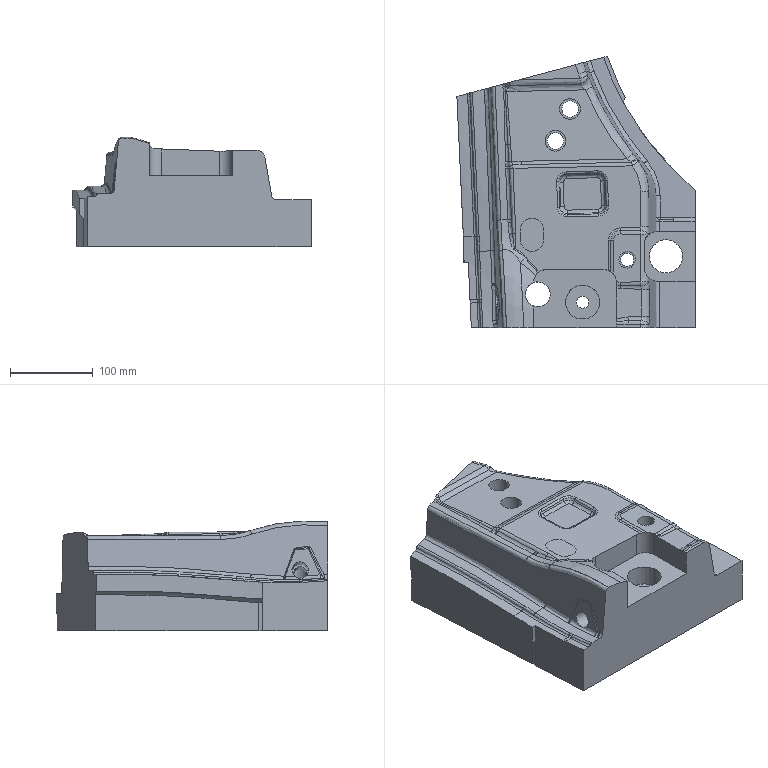Part | NX | features solid 2 | 1 solid | 204 faces | box 287.588 x 327.838 x 132.789 mm | volume 6916265 mm3 | spline 165 | plane 23 | cylinder 16 | commonest cylinder face diameters 30 x5 20 x4 16 x2 25 x2 15 x1 40 x1